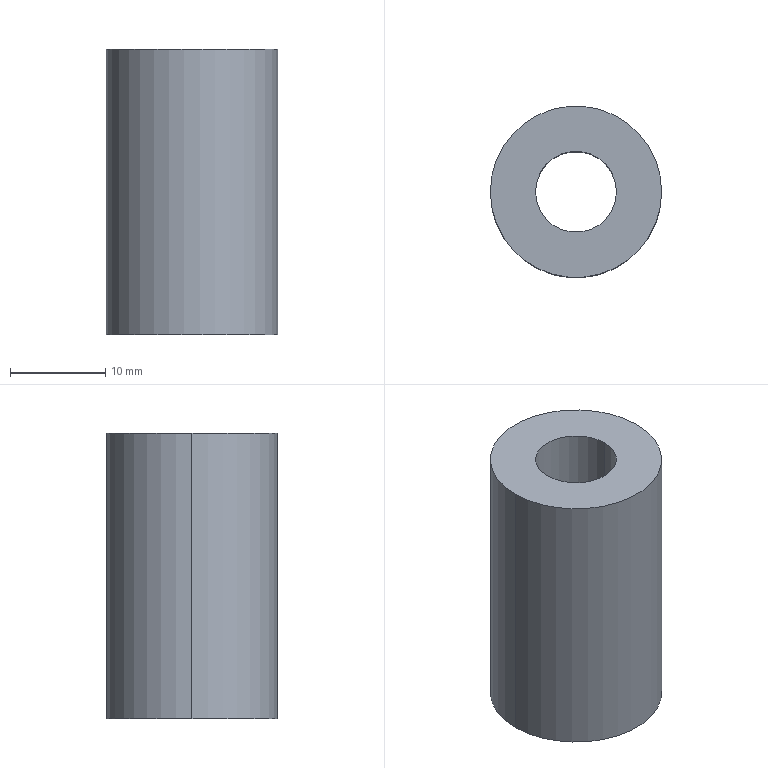Part | STEP file | 1 solid | 6 faces | box 18 x 18 x 30 mm | volume 5932 mm3 | cylinder 4 | plane 2 | commonest cylinder face diameters 8.5 x2 18 x2
STEP:
#1=CARTESIAN_POINT('',(0.,0.,0.));
#2=DIRECTION('',(0.,0.,1.));
#3=DIRECTION('',(1.,0.,0.));
#4=AXIS2_PLACEMENT_3D('',#1,#2,#3);
#5=CARTESIAN_POINT('',(9.,0.,0.));
#6=VERTEX_POINT('',#5);
#7=CARTESIAN_POINT('',(-9.,0.,0.));
#8=VERTEX_POINT('',#7);
#9=CARTESIAN_POINT('',(0.,0.,0.));
#10=DIRECTION('',(0.,0.,1.));
#11=DIRECTION('',(1.,0.,0.));
#12=AXIS2_PLACEMENT_3D('',#9,#10,#11);
#13=CIRCLE('',#12,9.);
#14=CARTESIAN_POINT('',(0.,0.,30.));
#15=DIRECTION('',(0.,0.,1.));
#16=DIRECTION('',(1.,0.,0.));
#17=AXIS2_PLACEMENT_3D('',#14,#15,#16);
#18=CYLINDRICAL_SURFACE('',#17,9.);
#19=CARTESIAN_POINT('',(0.,-30.));
#20=DIRECTION('',(1.,0.));
#21=VECTOR('',#20,1.);
#22=LINE('',#19,#21);
#23=(GEOMETRIC_REPRESENTATION_CONTEXT(2)PARAMETRIC_REPRESENTATION_CONTEXT()REPRESENTATION_CONTEXT('',''));
#24=DEFINITIONAL_REPRESENTATION('',(#22),#23);
#25=PCURVE('',#18,#24);
#26=CARTESIAN_POINT('',(0.,0.,0.));
#27=DIRECTION('',(0.,0.,1.));
#28=DIRECTION('',(1.,0.,0.));
#29=AXIS2_PLACEMENT_3D('',#26,#27,#28);
#30=PLANE('',#29);
#31=CARTESIAN_POINT('',(0.,0.));
#32=DIRECTION('',(1.,0.));
#33=AXIS2_PLACEMENT_2D('',#31,#32);
#34=CIRCLE('',#33,9.);
#35=(GEOMETRIC_REPRESENTATION_CONTEXT(2)PARAMETRIC_REPRESENTATION_CONTEXT()REPRESENTATION_CONTEXT('',''));
#36=DEFINITIONAL_REPRESENTATION('',(#34),#35);
#37=PCURVE('',#30,#36);
#38=SURFACE_CURVE('',#13,(#25,#37),.PCURVE_S1.);
#39=EDGE_CURVE('',#6,#8,#38,.T.);
#40=ORIENTED_EDGE('',*,*,#39,.T.);
#41=CARTESIAN_POINT('',(-9.,0.,30.));
#42=VERTEX_POINT('',#41);
#43=CARTESIAN_POINT('',(-9.,0.,30.));
#44=DIRECTION('',(0.,0.,1.));
#45=VECTOR('',#44,1.);
#46=LINE('',#43,#45);
#47=CARTESIAN_POINT('',(3.142,0.));
#48=DIRECTION('',(0.,1.));
#49=VECTOR('',#48,1.);
#50=LINE('',#47,#49);
#51=(GEOMETRIC_REPRESENTATION_CONTEXT(2)PARAMETRIC_REPRESENTATION_CONTEXT()REPRESENTATION_CONTEXT('',''));
#52=DEFINITIONAL_REPRESENTATION('',(#50),#51);
#53=PCURVE('',#18,#52);
#54=CARTESIAN_POINT('',(0.,0.,30.));
#55=DIRECTION('',(0.,0.,1.));
#56=DIRECTION('',(1.,0.,0.));
#57=AXIS2_PLACEMENT_3D('',#54,#55,#56);
#58=CYLINDRICAL_SURFACE('',#57,9.);
#59=CARTESIAN_POINT('',(3.142,0.));
#60=DIRECTION('',(0.,1.));
#61=VECTOR('',#60,1.);
#62=LINE('',#59,#61);
#63=(GEOMETRIC_REPRESENTATION_CONTEXT(2)PARAMETRIC_REPRESENTATION_CONTEXT()REPRESENTATION_CONTEXT('',''));
#64=DEFINITIONAL_REPRESENTATION('',(#62),#63);
#65=PCURVE('',#58,#64);
#66=SURFACE_CURVE('',#46,(#53,#65),.PCURVE_S1.);
#67=EDGE_CURVE('',#8,#42,#66,.T.);
#68=ORIENTED_EDGE('',*,*,#67,.T.);
#69=CARTESIAN_POINT('',(9.,0.,30.));
#70=VERTEX_POINT('',#69);
#71=CARTESIAN_POINT('',(0.,0.,30.));
#72=DIRECTION('',(0.,0.,-1.));
#73=DIRECTION('',(1.,0.,0.));
#74=AXIS2_PLACEMENT_3D('',#71,#72,#73);
#75=CIRCLE('',#74,9.);
#76=CARTESIAN_POINT('',(6.283,0.));
#77=DIRECTION('',(-1.,0.));
#78=VECTOR('',#77,1.);
#79=LINE('',#76,#78);
#80=(GEOMETRIC_REPRESENTATION_CONTEXT(2)PARAMETRIC_REPRESENTATION_CONTEXT()REPRESENTATION_CONTEXT('',''));
#81=DEFINITIONAL_REPRESENTATION('',(#79),#80);
#82=PCURVE('',#18,#81);
#83=CARTESIAN_POINT('',(0.,0.,30.));
#84=DIRECTION('',(0.,0.,1.));
#85=DIRECTION('',(1.,0.,0.));
#86=AXIS2_PLACEMENT_3D('',#83,#84,#85);
#87=PLANE('',#86);
#88=CARTESIAN_POINT('',(9.,0.));
#89=CARTESIAN_POINT('',(9.,-15.588));
#90=CARTESIAN_POINT('',(-4.5,-7.794));
#91=CARTESIAN_POINT('',(-18.,0.));
#92=CARTESIAN_POINT('',(-4.5,7.794));
#93=CARTESIAN_POINT('',(9.,15.588));
#94=CARTESIAN_POINT('',(9.,0.));
#95=(BOUNDED_CURVE()B_SPLINE_CURVE(2,(#88,#89,#90,#91,#92,#93,#94),.UNSPECIFIED.,.T.,.F.)B_SPLINE_CURVE_WITH_KNOTS((1,2,2,2,2,1),(-2.094,0.,2.094,4.189,6.283,8.378),.UNSPECIFIED.)CURVE()GEOMETRIC_REPRESENTATION_ITEM()RATIONAL_B_SPLINE_CURVE((1.,0.5,1.,0.5,1.,0.5,1.))REPRESENTATION_ITEM(''));
#96=(GEOMETRIC_REPRESENTATION_CONTEXT(2)PARAMETRIC_REPRESENTATION_CONTEXT()REPRESENTATION_CONTEXT('',''));
#97=DEFINITIONAL_REPRESENTATION('',(#95),#96);
#98=PCURVE('',#87,#97);
#99=SURFACE_CURVE('',#75,(#82,#98),.PCURVE_S1.);
#100=EDGE_CURVE('',#42,#70,#99,.T.);
#101=ORIENTED_EDGE('',*,*,#100,.T.);
#102=CARTESIAN_POINT('',(9.,0.,30.));
#103=DIRECTION('',(0.,0.,1.));
#104=VECTOR('',#103,1.);
#105=LINE('',#102,#104);
#106=CARTESIAN_POINT('',(0.,0.));
#107=DIRECTION('',(0.,1.));
#108=VECTOR('',#107,1.);
#109=LINE('',#106,#108);
#110=(GEOMETRIC_REPRESENTATION_CONTEXT(2)PARAMETRIC_REPRESENTATION_CONTEXT()REPRESENTATION_CONTEXT('',''));
#111=DEFINITIONAL_REPRESENTATION('',(#109),#110);
#112=PCURVE('',#18,#111);
#113=CARTESIAN_POINT('',(6.283,0.));
#114=DIRECTION('',(0.,1.));
#115=VECTOR('',#114,1.);
#116=LINE('',#113,#115);
#117=(GEOMETRIC_REPRESENTATION_CONTEXT(2)PARAMETRIC_REPRESENTATION_CONTEXT()REPRESENTATION_CONTEXT('',''));
#118=DEFINITIONAL_REPRESENTATION('',(#116),#117);
#119=PCURVE('',#58,#118);
#120=SURFACE_CURVE('',#105,(#112,#119),.PCURVE_S1.);
#121=EDGE_CURVE('',#6,#70,#120,.T.);
#122=ORIENTED_EDGE('',*,*,#121,.F.);
#123=EDGE_LOOP('',(#40,#68,#101,#122));
#124=FACE_BOUND('',#123,.T.);
#125=ADVANCED_FACE('',(#124),#18,.T.);
#126=CARTESIAN_POINT('',(4.25,0.,0.));
#127=VERTEX_POINT('',#126);
#128=CARTESIAN_POINT('',(4.25,0.,30.));
#129=VERTEX_POINT('',#128);
#130=CARTESIAN_POINT('',(4.25,0.,30.));
#131=DIRECTION('',(0.,0.,1.));
#132=VECTOR('',#131,1.);
#133=LINE('',#130,#132);
#134=CARTESIAN_POINT('',(0.,0.,30.));
#135=DIRECTION('',(0.,0.,1.));
#136=DIRECTION('',(1.,0.,0.));
#137=AXIS2_PLACEMENT_3D('',#134,#135,#136);
#138=CYLINDRICAL_SURFACE('',#137,4.25);
#139=CARTESIAN_POINT('',(6.283,0.));
#140=DIRECTION('',(0.,1.));
#141=VECTOR('',#140,1.);
#142=LINE('',#139,#141);
#143=(GEOMETRIC_REPRESENTATION_CONTEXT(2)PARAMETRIC_REPRESENTATION_CONTEXT()REPRESENTATION_CONTEXT('',''));
#144=DEFINITIONAL_REPRESENTATION('',(#142),#143);
#145=PCURVE('',#138,#144);
#146=CARTESIAN_POINT('',(0.,0.,30.));
#147=DIRECTION('',(0.,0.,1.));
#148=DIRECTION('',(1.,0.,0.));
#149=AXIS2_PLACEMENT_3D('',#146,#147,#148);
#150=CYLINDRICAL_SURFACE('',#149,4.25);
#151=CARTESIAN_POINT('',(0.,0.));
#152=DIRECTION('',(0.,1.));
#153=VECTOR('',#152,1.);
#154=LINE('',#151,#153);
#155=(GEOMETRIC_REPRESENTATION_CONTEXT(2)PARAMETRIC_REPRESENTATION_CONTEXT()REPRESENTATION_CONTEXT('',''));
#156=DEFINITIONAL_REPRESENTATION('',(#154),#155);
#157=PCURVE('',#150,#156);
#158=SURFACE_CURVE('',#133,(#145,#157),.PCURVE_S1.);
#159=EDGE_CURVE('',#127,#129,#158,.T.);
#160=ORIENTED_EDGE('',*,*,#159,.T.);
#161=CARTESIAN_POINT('',(-4.25,0.,30.));
#162=VERTEX_POINT('',#161);
#163=CARTESIAN_POINT('',(0.,0.,30.));
#164=DIRECTION('',(0.,0.,-1.));
#165=DIRECTION('',(1.,0.,0.));
#166=AXIS2_PLACEMENT_3D('',#163,#164,#165);
#167=CIRCLE('',#166,4.25);
#168=CARTESIAN_POINT('',(6.283,0.));
#169=DIRECTION('',(-1.,0.));
#170=VECTOR('',#169,1.);
#171=LINE('',#168,#170);
#172=(GEOMETRIC_REPRESENTATION_CONTEXT(2)PARAMETRIC_REPRESENTATION_CONTEXT()REPRESENTATION_CONTEXT('',''));
#173=DEFINITIONAL_REPRESENTATION('',(#171),#172);
#174=PCURVE('',#138,#173);
#175=CARTESIAN_POINT('',(4.25,0.));
#176=CARTESIAN_POINT('',(4.25,-7.361));
#177=CARTESIAN_POINT('',(-2.125,-3.681));
#178=CARTESIAN_POINT('',(-8.5,0.));
#179=CARTESIAN_POINT('',(-2.125,3.681));
#180=CARTESIAN_POINT('',(4.25,7.361));
#181=CARTESIAN_POINT('',(4.25,0.));
#182=(BOUNDED_CURVE()B_SPLINE_CURVE(2,(#175,#176,#177,#178,#179,#180,#181),.UNSPECIFIED.,.T.,.F.)B_SPLINE_CURVE_WITH_KNOTS((1,2,2,2,2,1),(-2.094,0.,2.094,4.189,6.283,8.378),.UNSPECIFIED.)CURVE()GEOMETRIC_REPRESENTATION_ITEM()RATIONAL_B_SPLINE_CURVE((1.,0.5,1.,0.5,1.,0.5,1.))REPRESENTATION_ITEM(''));
#183=(GEOMETRIC_REPRESENTATION_CONTEXT(2)PARAMETRIC_REPRESENTATION_CONTEXT()REPRESENTATION_CONTEXT('',''));
#184=DEFINITIONAL_REPRESENTATION('',(#182),#183);
#185=PCURVE('',#87,#184);
#186=SURFACE_CURVE('',#167,(#174,#185),.PCURVE_S1.);
#187=EDGE_CURVE('',#129,#162,#186,.T.);
#188=ORIENTED_EDGE('',*,*,#187,.T.);
#189=CARTESIAN_POINT('',(-4.25,0.,0.));
#190=VERTEX_POINT('',#189);
#191=CARTESIAN_POINT('',(-4.25,0.,30.));
#192=DIRECTION('',(0.,0.,1.));
#193=VECTOR('',#192,1.);
#194=LINE('',#191,#193);
#195=CARTESIAN_POINT('',(3.142,0.));
#196=DIRECTION('',(0.,1.));
#197=VECTOR('',#196,1.);
#198=LINE('',#195,#197);
#199=(GEOMETRIC_REPRESENTATION_CONTEXT(2)PARAMETRIC_REPRESENTATION_CONTEXT()REPRESENTATION_CONTEXT('',''));
#200=DEFINITIONAL_REPRESENTATION('',(#198),#199);
#201=PCURVE('',#138,#200);
#202=CARTESIAN_POINT('',(3.142,0.));
#203=DIRECTION('',(0.,1.));
#204=VECTOR('',#203,1.);
#205=LINE('',#202,#204);
#206=(GEOMETRIC_REPRESENTATION_CONTEXT(2)PARAMETRIC_REPRESENTATION_CONTEXT()REPRESENTATION_CONTEXT('',''));
#207=DEFINITIONAL_REPRESENTATION('',(#205),#206);
#208=PCURVE('',#150,#207);
#209=SURFACE_CURVE('',#194,(#201,#208),.PCURVE_S1.);
#210=EDGE_CURVE('',#190,#162,#209,.T.);
#211=ORIENTED_EDGE('',*,*,#210,.F.);
#212=CARTESIAN_POINT('',(0.,0.,0.));
#213=DIRECTION('',(0.,0.,-1.));
#214=DIRECTION('',(1.,0.,0.));
#215=AXIS2_PLACEMENT_3D('',#212,#213,#214);
#216=CIRCLE('',#215,4.25);
#217=CARTESIAN_POINT('',(6.283,-30.));
#218=DIRECTION('',(-1.,0.));
#219=VECTOR('',#218,1.);
#220=LINE('',#217,#219);
#221=(GEOMETRIC_REPRESENTATION_CONTEXT(2)PARAMETRIC_REPRESENTATION_CONTEXT()REPRESENTATION_CONTEXT('',''));
#222=DEFINITIONAL_REPRESENTATION('',(#220),#221);
#223=PCURVE('',#138,#222);
#224=CARTESIAN_POINT('',(4.25,0.));
#225=CARTESIAN_POINT('',(4.25,-7.361));
#226=CARTESIAN_POINT('',(-2.125,-3.681));
#227=CARTESIAN_POINT('',(-8.5,0.));
#228=CARTESIAN_POINT('',(-2.125,3.681));
#229=CARTESIAN_POINT('',(4.25,7.361));
#230=CARTESIAN_POINT('',(4.25,0.));
#231=(BOUNDED_CURVE()B_SPLINE_CURVE(2,(#224,#225,#226,#227,#228,#229,#230),.UNSPECIFIED.,.T.,.F.)B_SPLINE_CURVE_WITH_KNOTS((1,2,2,2,2,1),(-2.094,0.,2.094,4.189,6.283,8.378),.UNSPECIFIED.)CURVE()GEOMETRIC_REPRESENTATION_ITEM()RATIONAL_B_SPLINE_CURVE((1.,0.5,1.,0.5,1.,0.5,1.))REPRESENTATION_ITEM(''));
#232=(GEOMETRIC_REPRESENTATION_CONTEXT(2)PARAMETRIC_REPRESENTATION_CONTEXT()REPRESENTATION_CONTEXT('',''));
#233=DEFINITIONAL_REPRESENTATION('',(#231),#232);
#234=PCURVE('',#30,#233);
#235=SURFACE_CURVE('',#216,(#223,#234),.PCURVE_S1.);
#236=EDGE_CURVE('',#127,#190,#235,.T.);
#237=ORIENTED_EDGE('',*,*,#236,.F.);
#238=EDGE_LOOP('',(#160,#188,#211,#237));
#239=FACE_BOUND('',#238,.F.);
#240=ADVANCED_FACE('',(#239),#138,.F.);
#241=ORIENTED_EDGE('',*,*,#67,.F.);
#242=CARTESIAN_POINT('',(0.,0.,0.));
#243=DIRECTION('',(0.,0.,1.));
#244=DIRECTION('',(1.,0.,0.));
#245=AXIS2_PLACEMENT_3D('',#242,#243,#244);
#246=CIRCLE('',#245,9.);
#247=CARTESIAN_POINT('',(0.,-30.));
#248=DIRECTION('',(1.,0.));
#249=VECTOR('',#248,1.);
#250=LINE('',#247,#249);
#251=(GEOMETRIC_REPRESENTATION_CONTEXT(2)PARAMETRIC_REPRESENTATION_CONTEXT()REPRESENTATION_CONTEXT('',''));
#252=DEFINITIONAL_REPRESENTATION('',(#250),#251);
#253=PCURVE('',#58,#252);
#254=CARTESIAN_POINT('',(0.,0.));
#255=DIRECTION('',(1.,0.));
#256=AXIS2_PLACEMENT_2D('',#254,#255);
#257=CIRCLE('',#256,9.);
#258=(GEOMETRIC_REPRESENTATION_CONTEXT(2)PARAMETRIC_REPRESENTATION_CONTEXT()REPRESENTATION_CONTEXT('',''));
#259=DEFINITIONAL_REPRESENTATION('',(#257),#258);
#260=PCURVE('',#30,#259);
#261=SURFACE_CURVE('',#246,(#253,#260),.PCURVE_S1.);
#262=EDGE_CURVE('',#8,#6,#261,.T.);
#263=ORIENTED_EDGE('',*,*,#262,.T.);
#264=ORIENTED_EDGE('',*,*,#121,.T.);
#265=CARTESIAN_POINT('',(0.,0.,30.));
#266=DIRECTION('',(0.,0.,-1.));
#267=DIRECTION('',(1.,0.,0.));
#268=AXIS2_PLACEMENT_3D('',#265,#266,#267);
#269=CIRCLE('',#268,9.);
#270=CARTESIAN_POINT('',(6.283,0.));
#271=DIRECTION('',(-1.,0.));
#272=VECTOR('',#271,1.);
#273=LINE('',#270,#272);
#274=(GEOMETRIC_REPRESENTATION_CONTEXT(2)PARAMETRIC_REPRESENTATION_CONTEXT()REPRESENTATION_CONTEXT('',''));
#275=DEFINITIONAL_REPRESENTATION('',(#273),#274);
#276=PCURVE('',#58,#275);
#277=CARTESIAN_POINT('',(9.,0.));
#278=CARTESIAN_POINT('',(9.,-15.588));
#279=CARTESIAN_POINT('',(-4.5,-7.794));
#280=CARTESIAN_POINT('',(-18.,0.));
#281=CARTESIAN_POINT('',(-4.5,7.794));
#282=CARTESIAN_POINT('',(9.,15.588));
#283=CARTESIAN_POINT('',(9.,0.));
#284=(BOUNDED_CURVE()B_SPLINE_CURVE(2,(#277,#278,#279,#280,#281,#282,#283),.UNSPECIFIED.,.T.,.F.)B_SPLINE_CURVE_WITH_KNOTS((1,2,2,2,2,1),(-2.094,0.,2.094,4.189,6.283,8.378),.UNSPECIFIED.)CURVE()GEOMETRIC_REPRESENTATION_ITEM()RATIONAL_B_SPLINE_CURVE((1.,0.5,1.,0.5,1.,0.5,1.))REPRESENTATION_ITEM(''));
#285=(GEOMETRIC_REPRESENTATION_CONTEXT(2)PARAMETRIC_REPRESENTATION_CONTEXT()REPRESENTATION_CONTEXT('',''));
#286=DEFINITIONAL_REPRESENTATION('',(#284),#285);
#287=PCURVE('',#87,#286);
#288=SURFACE_CURVE('',#269,(#276,#287),.PCURVE_S1.);
#289=EDGE_CURVE('',#70,#42,#288,.T.);
#290=ORIENTED_EDGE('',*,*,#289,.T.);
#291=EDGE_LOOP('',(#241,#263,#264,#290));
#292=FACE_BOUND('',#291,.T.);
#293=ADVANCED_FACE('',(#292),#58,.T.);
#294=ORIENTED_EDGE('',*,*,#236,.F.);
#295=CARTESIAN_POINT('',(0.,0.,0.));
#296=DIRECTION('',(0.,0.,-1.));
#297=DIRECTION('',(1.,0.,0.));
#298=AXIS2_PLACEMENT_3D('',#295,#296,#297);
#299=CIRCLE('',#298,4.25);
#300=CARTESIAN_POINT('',(4.25,0.));
#301=CARTESIAN_POINT('',(4.25,-7.361));
#302=CARTESIAN_POINT('',(-2.125,-3.681));
#303=CARTESIAN_POINT('',(-8.5,0.));
#304=CARTESIAN_POINT('',(-2.125,3.681));
#305=CARTESIAN_POINT('',(4.25,7.361));
#306=CARTESIAN_POINT('',(4.25,0.));
#307=(BOUNDED_CURVE()B_SPLINE_CURVE(2,(#300,#301,#302,#303,#304,#305,#306),.UNSPECIFIED.,.T.,.F.)B_SPLINE_CURVE_WITH_KNOTS((1,2,2,2,2,1),(-2.094,0.,2.094,4.189,6.283,8.378),.UNSPECIFIED.)CURVE()GEOMETRIC_REPRESENTATION_ITEM()RATIONAL_B_SPLINE_CURVE((1.,0.5,1.,0.5,1.,0.5,1.))REPRESENTATION_ITEM(''));
#308=(GEOMETRIC_REPRESENTATION_CONTEXT(2)PARAMETRIC_REPRESENTATION_CONTEXT()REPRESENTATION_CONTEXT('',''));
#309=DEFINITIONAL_REPRESENTATION('',(#307),#308);
#310=PCURVE('',#30,#309);
#311=CARTESIAN_POINT('',(6.283,-30.));
#312=DIRECTION('',(-1.,0.));
#313=VECTOR('',#312,1.);
#314=LINE('',#311,#313);
#315=(GEOMETRIC_REPRESENTATION_CONTEXT(2)PARAMETRIC_REPRESENTATION_CONTEXT()REPRESENTATION_CONTEXT('',''));
#316=DEFINITIONAL_REPRESENTATION('',(#314),#315);
#317=PCURVE('',#150,#316);
#318=SURFACE_CURVE('',#299,(#310,#317),.PCURVE_S1.);
#319=EDGE_CURVE('',#190,#127,#318,.T.);
#320=ORIENTED_EDGE('',*,*,#319,.F.);
#321=EDGE_LOOP('',(#294,#320));
#322=FACE_BOUND('',#321,.T.);
#323=ORIENTED_EDGE('',*,*,#39,.F.);
#324=ORIENTED_EDGE('',*,*,#262,.F.);
#325=EDGE_LOOP('',(#323,#324));
#326=FACE_BOUND('',#325,.T.);
#327=ADVANCED_FACE('',(#322,#326),#30,.F.);
#328=ORIENTED_EDGE('',*,*,#187,.T.);
#329=CARTESIAN_POINT('',(0.,0.,30.));
#330=DIRECTION('',(0.,0.,-1.));
#331=DIRECTION('',(1.,0.,0.));
#332=AXIS2_PLACEMENT_3D('',#329,#330,#331);
#333=CIRCLE('',#332,4.25);
#334=CARTESIAN_POINT('',(4.25,0.));
#335=CARTESIAN_POINT('',(4.25,-7.361));
#336=CARTESIAN_POINT('',(-2.125,-3.681));
#337=CARTESIAN_POINT('',(-8.5,0.));
#338=CARTESIAN_POINT('',(-2.125,3.681));
#339=CARTESIAN_POINT('',(4.25,7.361));
#340=CARTESIAN_POINT('',(4.25,0.));
#341=(BOUNDED_CURVE()B_SPLINE_CURVE(2,(#334,#335,#336,#337,#338,#339,#340),.UNSPECIFIED.,.T.,.F.)B_SPLINE_CURVE_WITH_KNOTS((1,2,2,2,2,1),(-2.094,0.,2.094,4.189,6.283,8.378),.UNSPECIFIED.)CURVE()GEOMETRIC_REPRESENTATION_ITEM()RATIONAL_B_SPLINE_CURVE((1.,0.5,1.,0.5,1.,0.5,1.))REPRESENTATION_ITEM(''));
#342=(GEOMETRIC_REPRESENTATION_CONTEXT(2)PARAMETRIC_REPRESENTATION_CONTEXT()REPRESENTATION_CONTEXT('',''));
#343=DEFINITIONAL_REPRESENTATION('',(#341),#342);
#344=PCURVE('',#87,#343);
#345=CARTESIAN_POINT('',(6.283,0.));
#346=DIRECTION('',(-1.,0.));
#347=VECTOR('',#346,1.);
#348=LINE('',#345,#347);
#349=(GEOMETRIC_REPRESENTATION_CONTEXT(2)PARAMETRIC_REPRESENTATION_CONTEXT()REPRESENTATION_CONTEXT('',''));
#350=DEFINITIONAL_REPRESENTATION('',(#348),#349);
#351=PCURVE('',#150,#350);
#352=SURFACE_CURVE('',#333,(#344,#351),.PCURVE_S1.);
#353=EDGE_CURVE('',#162,#129,#352,.T.);
#354=ORIENTED_EDGE('',*,*,#353,.T.);
#355=EDGE_LOOP('',(#328,#354));
#356=FACE_BOUND('',#355,.T.);
#357=ORIENTED_EDGE('',*,*,#289,.F.);
#358=ORIENTED_EDGE('',*,*,#100,.F.);
#359=EDGE_LOOP('',(#357,#358));
#360=FACE_BOUND('',#359,.T.);
#361=ADVANCED_FACE('',(#356,#360),#87,.T.);
#362=ORIENTED_EDGE('',*,*,#353,.T.);
#363=ORIENTED_EDGE('',*,*,#159,.F.);
#364=ORIENTED_EDGE('',*,*,#319,.F.);
#365=ORIENTED_EDGE('',*,*,#210,.T.);
#366=EDGE_LOOP('',(#362,#363,#364,#365));
#367=FACE_BOUND('',#366,.F.);
#368=ADVANCED_FACE('',(#367),#150,.F.);
#369=CLOSED_SHELL('',(#125,#240,#293,#327,#361,#368));
#370=MANIFOLD_SOLID_BREP('',#369);
#371=(LENGTH_UNIT()NAMED_UNIT(*)SI_UNIT(.MILLI.,.METRE.));
#372=UNCERTAINTY_MEASURE_WITH_UNIT(LENGTH_MEASURE(0.0000001),#371,'','');
#373=(NAMED_UNIT(*)PLANE_ANGLE_UNIT()SI_UNIT($,.RADIAN.));
#374=(NAMED_UNIT(*)SI_UNIT($,.STERADIAN.)SOLID_ANGLE_UNIT());
#375=(GEOMETRIC_REPRESENTATION_CONTEXT(3)GLOBAL_UNCERTAINTY_ASSIGNED_CONTEXT((#372))GLOBAL_UNIT_ASSIGNED_CONTEXT((#371,#373,#374))REPRESENTATION_CONTEXT('',''));
#376=ADVANCED_BREP_SHAPE_REPRESENTATION('',(#4,#370),#375);